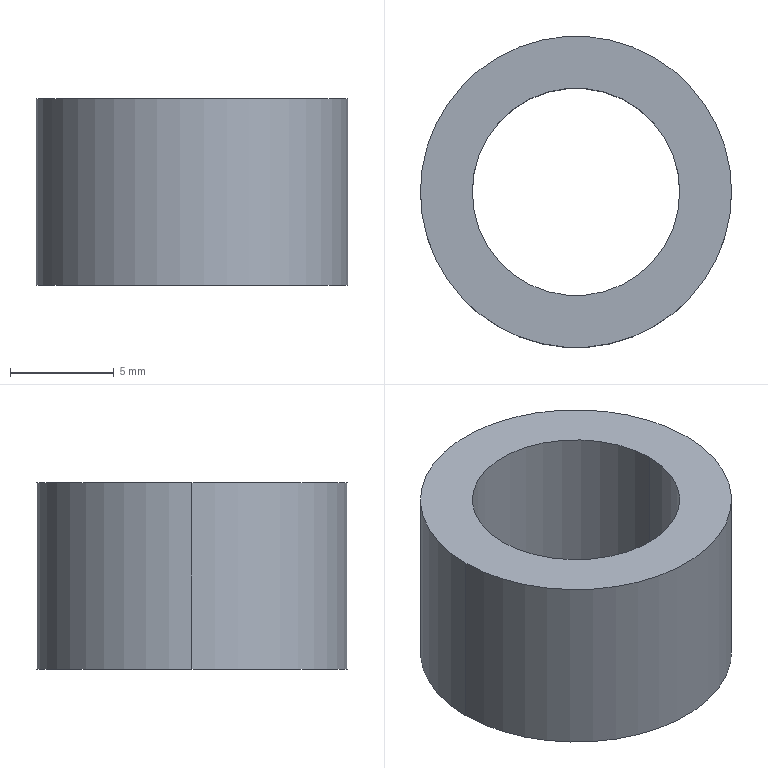Part | SolidWorks | features Extrusion 1 | 1 solid | 6 faces | box 15 x 15 x 9 mm | volume 883.573 mm3 | cylinder 4 | plane 2 | commonest cylinder face diameters 10 x2 15 x2
STEP:
#1=CARTESIAN_POINT('',(-5.,0.,9.));
#2=VERTEX_POINT('',#1);
#3=CARTESIAN_POINT('',(5.,0.,9.));
#4=VERTEX_POINT('',#3);
#5=CARTESIAN_POINT('',(0.,0.,9.));
#6=DIRECTION('',(0.,0.,1.));
#7=DIRECTION('',(1.,0.,0.));
#8=AXIS2_PLACEMENT_3D('',#5,#6,#7);
#9=CIRCLE('',#8,5.);
#10=EDGE_CURVE('',#2,#4,#9,.T.);
#11=ORIENTED_EDGE('',*,*,#10,.T.);
#12=CARTESIAN_POINT('',(5.,0.,0.));
#13=VERTEX_POINT('',#12);
#14=CARTESIAN_POINT('',(5.,0.,9.));
#15=DIRECTION('',(0.,0.,-1.));
#16=VECTOR('',#15,1000.);
#17=LINE('',#14,#16);
#18=EDGE_CURVE('',#4,#13,#17,.T.);
#19=ORIENTED_EDGE('',*,*,#18,.T.);
#20=CARTESIAN_POINT('',(-5.,0.,0.));
#21=VERTEX_POINT('',#20);
#22=CARTESIAN_POINT('',(0.,0.,0.));
#23=DIRECTION('',(0.,0.,1.));
#24=DIRECTION('',(1.,0.,0.));
#25=AXIS2_PLACEMENT_3D('',#22,#23,#24);
#26=CIRCLE('',#25,5.);
#27=EDGE_CURVE('',#21,#13,#26,.T.);
#28=ORIENTED_EDGE('',*,*,#27,.F.);
#29=CARTESIAN_POINT('',(-5.,0.,9.));
#30=DIRECTION('',(0.,0.,-1.));
#31=VECTOR('',#30,1000.);
#32=LINE('',#29,#31);
#33=EDGE_CURVE('',#2,#21,#32,.T.);
#34=ORIENTED_EDGE('',*,*,#33,.F.);
#35=EDGE_LOOP('',(#11,#19,#28,#34));
#36=FACE_OUTER_BOUND('',#35,.T.);
#37=CARTESIAN_POINT('',(0.,0.,9.));
#38=DIRECTION('',(0.,0.,-1.));
#39=DIRECTION('',(-1.,0.,0.));
#40=AXIS2_PLACEMENT_3D('',#37,#38,#39);
#41=CYLINDRICAL_SURFACE('',#40,5.);
#42=ADVANCED_FACE('',(#36),#41,.F.);
#43=CARTESIAN_POINT('',(7.5,0.,9.));
#44=VERTEX_POINT('',#43);
#45=CARTESIAN_POINT('',(-7.5,0.,9.));
#46=VERTEX_POINT('',#45);
#47=CARTESIAN_POINT('',(0.,0.,9.));
#48=DIRECTION('',(0.,0.,1.));
#49=DIRECTION('',(1.,0.,0.));
#50=AXIS2_PLACEMENT_3D('',#47,#48,#49);
#51=CIRCLE('',#50,7.5);
#52=EDGE_CURVE('',#44,#46,#51,.T.);
#53=ORIENTED_EDGE('',*,*,#52,.F.);
#54=CARTESIAN_POINT('',(7.5,0.,0.));
#55=VERTEX_POINT('',#54);
#56=CARTESIAN_POINT('',(7.5,0.,9.));
#57=DIRECTION('',(0.,0.,-1.));
#58=VECTOR('',#57,1000.);
#59=LINE('',#56,#58);
#60=EDGE_CURVE('',#44,#55,#59,.T.);
#61=ORIENTED_EDGE('',*,*,#60,.T.);
#62=CARTESIAN_POINT('',(-7.5,0.,0.));
#63=VERTEX_POINT('',#62);
#64=CARTESIAN_POINT('',(0.,0.,0.));
#65=DIRECTION('',(0.,0.,1.));
#66=DIRECTION('',(1.,0.,0.));
#67=AXIS2_PLACEMENT_3D('',#64,#65,#66);
#68=CIRCLE('',#67,7.5);
#69=EDGE_CURVE('',#55,#63,#68,.T.);
#70=ORIENTED_EDGE('',*,*,#69,.T.);
#71=CARTESIAN_POINT('',(-7.5,0.,9.));
#72=DIRECTION('',(0.,0.,-1.));
#73=VECTOR('',#72,1000.);
#74=LINE('',#71,#73);
#75=EDGE_CURVE('',#46,#63,#74,.T.);
#76=ORIENTED_EDGE('',*,*,#75,.F.);
#77=EDGE_LOOP('',(#53,#61,#70,#76));
#78=FACE_OUTER_BOUND('',#77,.T.);
#79=CARTESIAN_POINT('',(0.,0.,9.));
#80=DIRECTION('',(0.,0.,-1.));
#81=DIRECTION('',(-1.,0.,0.));
#82=AXIS2_PLACEMENT_3D('',#79,#80,#81);
#83=CYLINDRICAL_SURFACE('',#82,7.5);
#84=ADVANCED_FACE('',(#78),#83,.T.);
#85=CARTESIAN_POINT('',(0.,0.,9.));
#86=DIRECTION('',(0.,0.,1.));
#87=DIRECTION('',(1.,0.,0.));
#88=AXIS2_PLACEMENT_3D('',#85,#86,#87);
#89=CIRCLE('',#88,7.5);
#90=EDGE_CURVE('',#46,#44,#89,.T.);
#91=ORIENTED_EDGE('',*,*,#90,.T.);
#92=ORIENTED_EDGE('',*,*,#52,.T.);
#93=EDGE_LOOP('',(#91,#92));
#94=FACE_OUTER_BOUND('',#93,.T.);
#95=ORIENTED_EDGE('',*,*,#10,.F.);
#96=CARTESIAN_POINT('',(0.,0.,9.));
#97=DIRECTION('',(0.,0.,1.));
#98=DIRECTION('',(1.,0.,0.));
#99=AXIS2_PLACEMENT_3D('',#96,#97,#98);
#100=CIRCLE('',#99,5.);
#101=EDGE_CURVE('',#4,#2,#100,.T.);
#102=ORIENTED_EDGE('',*,*,#101,.F.);
#103=EDGE_LOOP('',(#95,#102));
#104=FACE_BOUND('',#103,.T.);
#105=CARTESIAN_POINT('',(0.,0.,9.));
#106=DIRECTION('',(0.,0.,1.));
#107=DIRECTION('',(1.,0.,0.));
#108=AXIS2_PLACEMENT_3D('',#105,#106,#107);
#109=PLANE('',#108);
#110=ADVANCED_FACE('',(#94,#104),#109,.T.);
#111=CARTESIAN_POINT('',(0.,0.,0.));
#112=DIRECTION('',(0.,0.,1.));
#113=DIRECTION('',(1.,0.,0.));
#114=AXIS2_PLACEMENT_3D('',#111,#112,#113);
#115=CIRCLE('',#114,7.5);
#116=EDGE_CURVE('',#63,#55,#115,.T.);
#117=ORIENTED_EDGE('',*,*,#116,.F.);
#118=ORIENTED_EDGE('',*,*,#69,.F.);
#119=EDGE_LOOP('',(#117,#118));
#120=FACE_OUTER_BOUND('',#119,.T.);
#121=ORIENTED_EDGE('',*,*,#27,.T.);
#122=CARTESIAN_POINT('',(0.,0.,0.));
#123=DIRECTION('',(0.,0.,1.));
#124=DIRECTION('',(1.,0.,0.));
#125=AXIS2_PLACEMENT_3D('',#122,#123,#124);
#126=CIRCLE('',#125,5.);
#127=EDGE_CURVE('',#13,#21,#126,.T.);
#128=ORIENTED_EDGE('',*,*,#127,.T.);
#129=EDGE_LOOP('',(#121,#128));
#130=FACE_BOUND('',#129,.T.);
#131=CARTESIAN_POINT('',(0.,0.,0.));
#132=DIRECTION('',(0.,0.,1.));
#133=DIRECTION('',(1.,0.,0.));
#134=AXIS2_PLACEMENT_3D('',#131,#132,#133);
#135=PLANE('',#134);
#136=ADVANCED_FACE('',(#120,#130),#135,.F.);
#137=ORIENTED_EDGE('',*,*,#60,.F.);
#138=ORIENTED_EDGE('',*,*,#90,.F.);
#139=ORIENTED_EDGE('',*,*,#75,.T.);
#140=ORIENTED_EDGE('',*,*,#116,.T.);
#141=EDGE_LOOP('',(#137,#138,#139,#140));
#142=FACE_OUTER_BOUND('',#141,.T.);
#143=CARTESIAN_POINT('',(0.,0.,9.));
#144=DIRECTION('',(0.,0.,-1.));
#145=DIRECTION('',(-1.,0.,0.));
#146=AXIS2_PLACEMENT_3D('',#143,#144,#145);
#147=CYLINDRICAL_SURFACE('',#146,7.5);
#148=ADVANCED_FACE('',(#142),#147,.T.);
#149=ORIENTED_EDGE('',*,*,#18,.F.);
#150=ORIENTED_EDGE('',*,*,#101,.T.);
#151=ORIENTED_EDGE('',*,*,#33,.T.);
#152=ORIENTED_EDGE('',*,*,#127,.F.);
#153=EDGE_LOOP('',(#149,#150,#151,#152));
#154=FACE_OUTER_BOUND('',#153,.T.);
#155=CARTESIAN_POINT('',(0.,0.,9.));
#156=DIRECTION('',(0.,0.,-1.));
#157=DIRECTION('',(-1.,0.,0.));
#158=AXIS2_PLACEMENT_3D('',#155,#156,#157);
#159=CYLINDRICAL_SURFACE('',#158,5.);
#160=ADVANCED_FACE('',(#154),#159,.F.);
#161=CLOSED_SHELL('',(#42,#84,#110,#136,#148,#160));
#162=MANIFOLD_SOLID_BREP('',#161);
#163=CARTESIAN_POINT('',(0.,0.,0.));
#164=DIRECTION('',(0.,0.,1.));
#165=DIRECTION('',(1.,0.,0.));
#166=AXIS2_PLACEMENT_3D('',#163,#164,#165);
#167=(LENGTH_UNIT()NAMED_UNIT(*)SI_UNIT(.MILLI.,.METRE.));
#168=UNCERTAINTY_MEASURE_WITH_UNIT(LENGTH_MEASURE(0.00001),#167,'','');
#169=(NAMED_UNIT(*)PLANE_ANGLE_UNIT()SI_UNIT($,.RADIAN.));
#170=(NAMED_UNIT(*)SI_UNIT($,.STERADIAN.)SOLID_ANGLE_UNIT());
#171=(GEOMETRIC_REPRESENTATION_CONTEXT(3)GLOBAL_UNCERTAINTY_ASSIGNED_CONTEXT((#168))GLOBAL_UNIT_ASSIGNED_CONTEXT((#167,#169,#170))REPRESENTATION_CONTEXT('',''));
#172=ADVANCED_BREP_SHAPE_REPRESENTATION('',(#162,#166),#171);